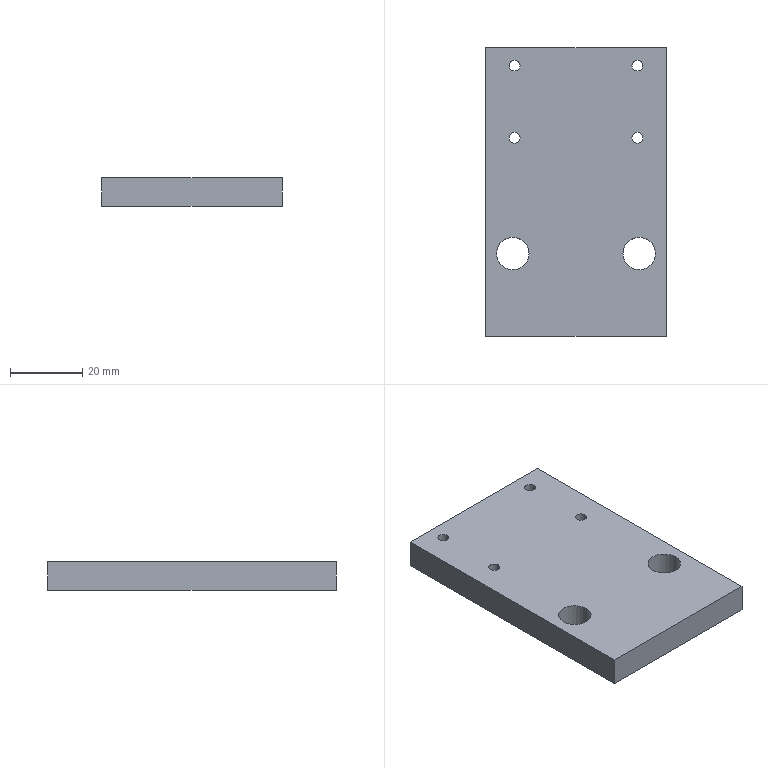Part | STEP file | X77b-01018 | 1 solid | 18 faces | box 50 x 80 x 8 mm | volume 30756 mm3 | cylinder 12 | plane 6 | commonest cylinder face diameters 3 x8 9 x4
STEP:
#1=CARTESIAN_POINT('',(54.163,-91.578,0.));
#2=VERTEX_POINT('',#1);
#3=CARTESIAN_POINT('',(57.163,-91.578,0.));
#4=VERTEX_POINT('',#3);
#5=CARTESIAN_POINT('',(55.663,-91.578,0.));
#6=DIRECTION('',(0.,0.,1.));
#7=DIRECTION('',(1.,0.,0.));
#8=AXIS2_PLACEMENT_3D('',#5,#6,#7);
#9=CIRCLE('',#8,1.5);
#10=EDGE_CURVE('',#2,#4,#9,.T.);
#11=ORIENTED_EDGE('',*,*,#10,.F.);
#12=CARTESIAN_POINT('',(54.163,-91.578,8.));
#13=VERTEX_POINT('',#12);
#14=CARTESIAN_POINT('',(54.163,-91.578,8.));
#15=DIRECTION('',(0.,0.,1.));
#16=VECTOR('',#15,1000.);
#17=LINE('',#14,#16);
#18=EDGE_CURVE('',#2,#13,#17,.T.);
#19=ORIENTED_EDGE('',*,*,#18,.T.);
#20=CARTESIAN_POINT('',(57.163,-91.578,8.));
#21=VERTEX_POINT('',#20);
#22=CARTESIAN_POINT('',(55.663,-91.578,8.));
#23=DIRECTION('',(0.,0.,1.));
#24=DIRECTION('',(1.,0.,0.));
#25=AXIS2_PLACEMENT_3D('',#22,#23,#24);
#26=CIRCLE('',#25,1.5);
#27=EDGE_CURVE('',#13,#21,#26,.T.);
#28=ORIENTED_EDGE('',*,*,#27,.T.);
#29=CARTESIAN_POINT('',(57.163,-91.578,8.));
#30=DIRECTION('',(0.,0.,1.));
#31=VECTOR('',#30,1000.);
#32=LINE('',#29,#31);
#33=EDGE_CURVE('',#4,#21,#32,.T.);
#34=ORIENTED_EDGE('',*,*,#33,.F.);
#35=EDGE_LOOP('',(#11,#19,#28,#34));
#36=FACE_OUTER_BOUND('',#35,.T.);
#37=CARTESIAN_POINT('',(55.663,-91.578,8.));
#38=DIRECTION('',(0.,0.,1.));
#39=DIRECTION('',(1.,0.,0.));
#40=AXIS2_PLACEMENT_3D('',#37,#38,#39);
#41=CYLINDRICAL_SURFACE('',#40,1.5);
#42=ADVANCED_FACE('',(#36),#41,.F.);
#43=CARTESIAN_POINT('',(54.163,-71.578,0.));
#44=VERTEX_POINT('',#43);
#45=CARTESIAN_POINT('',(57.163,-71.578,0.));
#46=VERTEX_POINT('',#45);
#47=CARTESIAN_POINT('',(55.663,-71.578,0.));
#48=DIRECTION('',(0.,0.,1.));
#49=DIRECTION('',(1.,0.,0.));
#50=AXIS2_PLACEMENT_3D('',#47,#48,#49);
#51=CIRCLE('',#50,1.5);
#52=EDGE_CURVE('',#44,#46,#51,.T.);
#53=ORIENTED_EDGE('',*,*,#52,.F.);
#54=CARTESIAN_POINT('',(54.163,-71.578,8.));
#55=VERTEX_POINT('',#54);
#56=CARTESIAN_POINT('',(54.163,-71.578,8.));
#57=DIRECTION('',(0.,0.,1.));
#58=VECTOR('',#57,1000.);
#59=LINE('',#56,#58);
#60=EDGE_CURVE('',#44,#55,#59,.T.);
#61=ORIENTED_EDGE('',*,*,#60,.T.);
#62=CARTESIAN_POINT('',(57.163,-71.578,8.));
#63=VERTEX_POINT('',#62);
#64=CARTESIAN_POINT('',(55.663,-71.578,8.));
#65=DIRECTION('',(0.,0.,1.));
#66=DIRECTION('',(1.,0.,0.));
#67=AXIS2_PLACEMENT_3D('',#64,#65,#66);
#68=CIRCLE('',#67,1.5);
#69=EDGE_CURVE('',#55,#63,#68,.T.);
#70=ORIENTED_EDGE('',*,*,#69,.T.);
#71=CARTESIAN_POINT('',(57.163,-71.578,8.));
#72=DIRECTION('',(0.,0.,1.));
#73=VECTOR('',#72,1000.);
#74=LINE('',#71,#73);
#75=EDGE_CURVE('',#46,#63,#74,.T.);
#76=ORIENTED_EDGE('',*,*,#75,.F.);
#77=EDGE_LOOP('',(#53,#61,#70,#76));
#78=FACE_OUTER_BOUND('',#77,.T.);
#79=CARTESIAN_POINT('',(55.663,-71.578,8.));
#80=DIRECTION('',(0.,0.,1.));
#81=DIRECTION('',(1.,0.,0.));
#82=AXIS2_PLACEMENT_3D('',#79,#80,#81);
#83=CYLINDRICAL_SURFACE('',#82,1.5);
#84=ADVANCED_FACE('',(#78),#83,.F.);
#85=CARTESIAN_POINT('',(88.163,-91.578,0.));
#86=VERTEX_POINT('',#85);
#87=CARTESIAN_POINT('',(91.163,-91.578,0.));
#88=VERTEX_POINT('',#87);
#89=CARTESIAN_POINT('',(89.663,-91.578,0.));
#90=DIRECTION('',(0.,0.,1.));
#91=DIRECTION('',(1.,0.,0.));
#92=AXIS2_PLACEMENT_3D('',#89,#90,#91);
#93=CIRCLE('',#92,1.5);
#94=EDGE_CURVE('',#86,#88,#93,.T.);
#95=ORIENTED_EDGE('',*,*,#94,.F.);
#96=CARTESIAN_POINT('',(88.163,-91.578,8.));
#97=VERTEX_POINT('',#96);
#98=CARTESIAN_POINT('',(88.163,-91.578,8.));
#99=DIRECTION('',(0.,0.,1.));
#100=VECTOR('',#99,1000.);
#101=LINE('',#98,#100);
#102=EDGE_CURVE('',#86,#97,#101,.T.);
#103=ORIENTED_EDGE('',*,*,#102,.T.);
#104=CARTESIAN_POINT('',(91.163,-91.578,8.));
#105=VERTEX_POINT('',#104);
#106=CARTESIAN_POINT('',(89.663,-91.578,8.));
#107=DIRECTION('',(0.,0.,1.));
#108=DIRECTION('',(1.,0.,0.));
#109=AXIS2_PLACEMENT_3D('',#106,#107,#108);
#110=CIRCLE('',#109,1.5);
#111=EDGE_CURVE('',#97,#105,#110,.T.);
#112=ORIENTED_EDGE('',*,*,#111,.T.);
#113=CARTESIAN_POINT('',(91.163,-91.578,8.));
#114=DIRECTION('',(0.,0.,1.));
#115=VECTOR('',#114,1000.);
#116=LINE('',#113,#115);
#117=EDGE_CURVE('',#88,#105,#116,.T.);
#118=ORIENTED_EDGE('',*,*,#117,.F.);
#119=EDGE_LOOP('',(#95,#103,#112,#118));
#120=FACE_OUTER_BOUND('',#119,.T.);
#121=CARTESIAN_POINT('',(89.663,-91.578,8.));
#122=DIRECTION('',(0.,0.,1.));
#123=DIRECTION('',(1.,0.,0.));
#124=AXIS2_PLACEMENT_3D('',#121,#122,#123);
#125=CYLINDRICAL_SURFACE('',#124,1.5);
#126=ADVANCED_FACE('',(#120),#125,.F.);
#127=CARTESIAN_POINT('',(88.163,-71.578,0.));
#128=VERTEX_POINT('',#127);
#129=CARTESIAN_POINT('',(91.163,-71.578,0.));
#130=VERTEX_POINT('',#129);
#131=CARTESIAN_POINT('',(89.663,-71.578,0.));
#132=DIRECTION('',(0.,0.,1.));
#133=DIRECTION('',(1.,0.,0.));
#134=AXIS2_PLACEMENT_3D('',#131,#132,#133);
#135=CIRCLE('',#134,1.5);
#136=EDGE_CURVE('',#128,#130,#135,.T.);
#137=ORIENTED_EDGE('',*,*,#136,.F.);
#138=CARTESIAN_POINT('',(88.163,-71.578,8.));
#139=VERTEX_POINT('',#138);
#140=CARTESIAN_POINT('',(88.163,-71.578,8.));
#141=DIRECTION('',(0.,0.,1.));
#142=VECTOR('',#141,1000.);
#143=LINE('',#140,#142);
#144=EDGE_CURVE('',#128,#139,#143,.T.);
#145=ORIENTED_EDGE('',*,*,#144,.T.);
#146=CARTESIAN_POINT('',(91.163,-71.578,8.));
#147=VERTEX_POINT('',#146);
#148=CARTESIAN_POINT('',(89.663,-71.578,8.));
#149=DIRECTION('',(0.,0.,1.));
#150=DIRECTION('',(1.,0.,0.));
#151=AXIS2_PLACEMENT_3D('',#148,#149,#150);
#152=CIRCLE('',#151,1.5);
#153=EDGE_CURVE('',#139,#147,#152,.T.);
#154=ORIENTED_EDGE('',*,*,#153,.T.);
#155=CARTESIAN_POINT('',(91.163,-71.578,8.));
#156=DIRECTION('',(0.,0.,1.));
#157=VECTOR('',#156,1000.);
#158=LINE('',#155,#157);
#159=EDGE_CURVE('',#130,#147,#158,.T.);
#160=ORIENTED_EDGE('',*,*,#159,.F.);
#161=EDGE_LOOP('',(#137,#145,#154,#160));
#162=FACE_OUTER_BOUND('',#161,.T.);
#163=CARTESIAN_POINT('',(89.663,-71.578,8.));
#164=DIRECTION('',(0.,0.,1.));
#165=DIRECTION('',(1.,0.,0.));
#166=AXIS2_PLACEMENT_3D('',#163,#164,#165);
#167=CYLINDRICAL_SURFACE('',#166,1.5);
#168=ADVANCED_FACE('',(#162),#167,.F.);
#169=CARTESIAN_POINT('',(85.663,-123.626,0.));
#170=VERTEX_POINT('',#169);
#171=CARTESIAN_POINT('',(94.663,-123.626,0.));
#172=VERTEX_POINT('',#171);
#173=CARTESIAN_POINT('',(90.163,-123.626,0.));
#174=DIRECTION('',(0.,0.,1.));
#175=DIRECTION('',(1.,0.,0.));
#176=AXIS2_PLACEMENT_3D('',#173,#174,#175);
#177=CIRCLE('',#176,4.5);
#178=EDGE_CURVE('',#170,#172,#177,.T.);
#179=ORIENTED_EDGE('',*,*,#178,.F.);
#180=CARTESIAN_POINT('',(85.663,-123.626,8.));
#181=VERTEX_POINT('',#180);
#182=CARTESIAN_POINT('',(85.663,-123.626,8.));
#183=DIRECTION('',(0.,0.,1.));
#184=VECTOR('',#183,1000.);
#185=LINE('',#182,#184);
#186=EDGE_CURVE('',#170,#181,#185,.T.);
#187=ORIENTED_EDGE('',*,*,#186,.T.);
#188=CARTESIAN_POINT('',(94.663,-123.626,8.));
#189=VERTEX_POINT('',#188);
#190=CARTESIAN_POINT('',(90.163,-123.626,8.));
#191=DIRECTION('',(0.,0.,1.));
#192=DIRECTION('',(1.,0.,0.));
#193=AXIS2_PLACEMENT_3D('',#190,#191,#192);
#194=CIRCLE('',#193,4.5);
#195=EDGE_CURVE('',#181,#189,#194,.T.);
#196=ORIENTED_EDGE('',*,*,#195,.T.);
#197=CARTESIAN_POINT('',(94.663,-123.626,8.));
#198=DIRECTION('',(0.,0.,1.));
#199=VECTOR('',#198,1000.);
#200=LINE('',#197,#199);
#201=EDGE_CURVE('',#172,#189,#200,.T.);
#202=ORIENTED_EDGE('',*,*,#201,.F.);
#203=EDGE_LOOP('',(#179,#187,#196,#202));
#204=FACE_OUTER_BOUND('',#203,.T.);
#205=CARTESIAN_POINT('',(90.163,-123.626,8.));
#206=DIRECTION('',(0.,0.,1.));
#207=DIRECTION('',(1.,0.,0.));
#208=AXIS2_PLACEMENT_3D('',#205,#206,#207);
#209=CYLINDRICAL_SURFACE('',#208,4.5);
#210=ADVANCED_FACE('',(#204),#209,.F.);
#211=CARTESIAN_POINT('',(50.663,-123.626,0.));
#212=VERTEX_POINT('',#211);
#213=CARTESIAN_POINT('',(59.663,-123.626,0.));
#214=VERTEX_POINT('',#213);
#215=CARTESIAN_POINT('',(55.163,-123.626,0.));
#216=DIRECTION('',(0.,0.,1.));
#217=DIRECTION('',(1.,0.,0.));
#218=AXIS2_PLACEMENT_3D('',#215,#216,#217);
#219=CIRCLE('',#218,4.5);
#220=EDGE_CURVE('',#212,#214,#219,.T.);
#221=ORIENTED_EDGE('',*,*,#220,.F.);
#222=CARTESIAN_POINT('',(50.663,-123.626,8.));
#223=VERTEX_POINT('',#222);
#224=CARTESIAN_POINT('',(50.663,-123.626,8.));
#225=DIRECTION('',(0.,0.,1.));
#226=VECTOR('',#225,1000.);
#227=LINE('',#224,#226);
#228=EDGE_CURVE('',#212,#223,#227,.T.);
#229=ORIENTED_EDGE('',*,*,#228,.T.);
#230=CARTESIAN_POINT('',(59.663,-123.626,8.));
#231=VERTEX_POINT('',#230);
#232=CARTESIAN_POINT('',(55.163,-123.626,8.));
#233=DIRECTION('',(0.,0.,1.));
#234=DIRECTION('',(1.,0.,0.));
#235=AXIS2_PLACEMENT_3D('',#232,#233,#234);
#236=CIRCLE('',#235,4.5);
#237=EDGE_CURVE('',#223,#231,#236,.T.);
#238=ORIENTED_EDGE('',*,*,#237,.T.);
#239=CARTESIAN_POINT('',(59.663,-123.626,8.));
#240=DIRECTION('',(0.,0.,1.));
#241=VECTOR('',#240,1000.);
#242=LINE('',#239,#241);
#243=EDGE_CURVE('',#214,#231,#242,.T.);
#244=ORIENTED_EDGE('',*,*,#243,.F.);
#245=EDGE_LOOP('',(#221,#229,#238,#244));
#246=FACE_OUTER_BOUND('',#245,.T.);
#247=CARTESIAN_POINT('',(55.163,-123.626,8.));
#248=DIRECTION('',(0.,0.,1.));
#249=DIRECTION('',(1.,0.,0.));
#250=AXIS2_PLACEMENT_3D('',#247,#248,#249);
#251=CYLINDRICAL_SURFACE('',#250,4.5);
#252=ADVANCED_FACE('',(#246),#251,.F.);
#253=CARTESIAN_POINT('',(47.663,-66.578,0.));
#254=VERTEX_POINT('',#253);
#255=CARTESIAN_POINT('',(47.663,-146.578,0.));
#256=VERTEX_POINT('',#255);
#257=CARTESIAN_POINT('',(47.663,-66.578,0.));
#258=DIRECTION('',(0.,-1.,0.));
#259=VECTOR('',#258,1000.);
#260=LINE('',#257,#259);
#261=EDGE_CURVE('',#254,#256,#260,.T.);
#262=ORIENTED_EDGE('',*,*,#261,.T.);
#263=CARTESIAN_POINT('',(47.663,-146.578,8.));
#264=VERTEX_POINT('',#263);
#265=CARTESIAN_POINT('',(47.663,-146.578,8.));
#266=DIRECTION('',(0.,0.,-1.));
#267=VECTOR('',#266,1000.);
#268=LINE('',#265,#267);
#269=EDGE_CURVE('',#264,#256,#268,.T.);
#270=ORIENTED_EDGE('',*,*,#269,.F.);
#271=CARTESIAN_POINT('',(47.663,-66.578,8.));
#272=VERTEX_POINT('',#271);
#273=CARTESIAN_POINT('',(47.663,-66.578,8.));
#274=DIRECTION('',(0.,-1.,0.));
#275=VECTOR('',#274,1000.);
#276=LINE('',#273,#275);
#277=EDGE_CURVE('',#272,#264,#276,.T.);
#278=ORIENTED_EDGE('',*,*,#277,.F.);
#279=CARTESIAN_POINT('',(47.663,-66.578,8.));
#280=DIRECTION('',(0.,0.,-1.));
#281=VECTOR('',#280,1000.);
#282=LINE('',#279,#281);
#283=EDGE_CURVE('',#272,#254,#282,.T.);
#284=ORIENTED_EDGE('',*,*,#283,.T.);
#285=EDGE_LOOP('',(#262,#270,#278,#284));
#286=FACE_OUTER_BOUND('',#285,.T.);
#287=CARTESIAN_POINT('',(47.663,-66.578,8.));
#288=DIRECTION('',(1.,0.,0.));
#289=DIRECTION('',(0.,1.,0.));
#290=AXIS2_PLACEMENT_3D('',#287,#288,#289);
#291=PLANE('',#290);
#292=ADVANCED_FACE('',(#286),#291,.F.);
#293=CARTESIAN_POINT('',(97.663,-146.578,0.));
#294=VERTEX_POINT('',#293);
#295=CARTESIAN_POINT('',(47.663,-146.578,0.));
#296=DIRECTION('',(1.,0.,0.));
#297=VECTOR('',#296,1000.);
#298=LINE('',#295,#297);
#299=EDGE_CURVE('',#256,#294,#298,.T.);
#300=ORIENTED_EDGE('',*,*,#299,.T.);
#301=CARTESIAN_POINT('',(97.663,-146.578,8.));
#302=VERTEX_POINT('',#301);
#303=CARTESIAN_POINT('',(97.663,-146.578,8.));
#304=DIRECTION('',(0.,0.,-1.));
#305=VECTOR('',#304,1000.);
#306=LINE('',#303,#305);
#307=EDGE_CURVE('',#302,#294,#306,.T.);
#308=ORIENTED_EDGE('',*,*,#307,.F.);
#309=CARTESIAN_POINT('',(47.663,-146.578,8.));
#310=DIRECTION('',(1.,0.,0.));
#311=VECTOR('',#310,1000.);
#312=LINE('',#309,#311);
#313=EDGE_CURVE('',#264,#302,#312,.T.);
#314=ORIENTED_EDGE('',*,*,#313,.F.);
#315=ORIENTED_EDGE('',*,*,#269,.T.);
#316=EDGE_LOOP('',(#300,#308,#314,#315));
#317=FACE_OUTER_BOUND('',#316,.T.);
#318=CARTESIAN_POINT('',(47.663,-146.578,8.));
#319=DIRECTION('',(0.,1.,0.));
#320=DIRECTION('',(0.,0.,1.));
#321=AXIS2_PLACEMENT_3D('',#318,#319,#320);
#322=PLANE('',#321);
#323=ADVANCED_FACE('',(#317),#322,.F.);
#324=CARTESIAN_POINT('',(97.663,-66.578,0.));
#325=VERTEX_POINT('',#324);
#326=CARTESIAN_POINT('',(97.663,-66.578,0.));
#327=DIRECTION('',(0.,1.,0.));
#328=VECTOR('',#327,1000.);
#329=LINE('',#326,#328);
#330=EDGE_CURVE('',#294,#325,#329,.T.);
#331=ORIENTED_EDGE('',*,*,#330,.T.);
#332=CARTESIAN_POINT('',(97.663,-66.578,8.));
#333=VERTEX_POINT('',#332);
#334=CARTESIAN_POINT('',(97.663,-66.578,8.));
#335=DIRECTION('',(0.,0.,-1.));
#336=VECTOR('',#335,1000.);
#337=LINE('',#334,#336);
#338=EDGE_CURVE('',#333,#325,#337,.T.);
#339=ORIENTED_EDGE('',*,*,#338,.F.);
#340=CARTESIAN_POINT('',(97.663,-66.578,8.));
#341=DIRECTION('',(0.,1.,0.));
#342=VECTOR('',#341,1000.);
#343=LINE('',#340,#342);
#344=EDGE_CURVE('',#302,#333,#343,.T.);
#345=ORIENTED_EDGE('',*,*,#344,.F.);
#346=ORIENTED_EDGE('',*,*,#307,.T.);
#347=EDGE_LOOP('',(#331,#339,#345,#346));
#348=FACE_OUTER_BOUND('',#347,.T.);
#349=CARTESIAN_POINT('',(97.663,-66.578,8.));
#350=DIRECTION('',(-1.,0.,0.));
#351=DIRECTION('',(0.,0.,1.));
#352=AXIS2_PLACEMENT_3D('',#349,#350,#351);
#353=PLANE('',#352);
#354=ADVANCED_FACE('',(#348),#353,.F.);
#355=CARTESIAN_POINT('',(47.663,-66.578,0.));
#356=DIRECTION('',(-1.,0.,0.));
#357=VECTOR('',#356,1000.);
#358=LINE('',#355,#357);
#359=EDGE_CURVE('',#325,#254,#358,.T.);
#360=ORIENTED_EDGE('',*,*,#359,.T.);
#361=ORIENTED_EDGE('',*,*,#283,.F.);
#362=CARTESIAN_POINT('',(47.663,-66.578,8.));
#363=DIRECTION('',(-1.,0.,0.));
#364=VECTOR('',#363,1000.);
#365=LINE('',#362,#364);
#366=EDGE_CURVE('',#333,#272,#365,.T.);
#367=ORIENTED_EDGE('',*,*,#366,.F.);
#368=ORIENTED_EDGE('',*,*,#338,.T.);
#369=EDGE_LOOP('',(#360,#361,#367,#368));
#370=FACE_OUTER_BOUND('',#369,.T.);
#371=CARTESIAN_POINT('',(47.663,-66.578,8.));
#372=DIRECTION('',(0.,-1.,0.));
#373=DIRECTION('',(0.,0.,-1.));
#374=AXIS2_PLACEMENT_3D('',#371,#372,#373);
#375=PLANE('',#374);
#376=ADVANCED_FACE('',(#370),#375,.F.);
#377=CARTESIAN_POINT('',(55.663,-91.578,8.));
#378=DIRECTION('',(0.,0.,1.));
#379=DIRECTION('',(1.,0.,0.));
#380=AXIS2_PLACEMENT_3D('',#377,#378,#379);
#381=CIRCLE('',#380,1.5);
#382=EDGE_CURVE('',#21,#13,#381,.T.);
#383=ORIENTED_EDGE('',*,*,#382,.F.);
#384=ORIENTED_EDGE('',*,*,#27,.F.);
#385=EDGE_LOOP('',(#383,#384));
#386=FACE_BOUND('',#385,.T.);
#387=CARTESIAN_POINT('',(55.663,-71.578,8.));
#388=DIRECTION('',(0.,0.,1.));
#389=DIRECTION('',(1.,0.,0.));
#390=AXIS2_PLACEMENT_3D('',#387,#388,#389);
#391=CIRCLE('',#390,1.5);
#392=EDGE_CURVE('',#63,#55,#391,.T.);
#393=ORIENTED_EDGE('',*,*,#392,.F.);
#394=ORIENTED_EDGE('',*,*,#69,.F.);
#395=EDGE_LOOP('',(#393,#394));
#396=FACE_BOUND('',#395,.T.);
#397=CARTESIAN_POINT('',(89.663,-91.578,8.));
#398=DIRECTION('',(0.,0.,1.));
#399=DIRECTION('',(1.,0.,0.));
#400=AXIS2_PLACEMENT_3D('',#397,#398,#399);
#401=CIRCLE('',#400,1.5);
#402=EDGE_CURVE('',#105,#97,#401,.T.);
#403=ORIENTED_EDGE('',*,*,#402,.F.);
#404=ORIENTED_EDGE('',*,*,#111,.F.);
#405=EDGE_LOOP('',(#403,#404));
#406=FACE_BOUND('',#405,.T.);
#407=CARTESIAN_POINT('',(89.663,-71.578,8.));
#408=DIRECTION('',(0.,0.,1.));
#409=DIRECTION('',(1.,0.,0.));
#410=AXIS2_PLACEMENT_3D('',#407,#408,#409);
#411=CIRCLE('',#410,1.5);
#412=EDGE_CURVE('',#147,#139,#411,.T.);
#413=ORIENTED_EDGE('',*,*,#412,.F.);
#414=ORIENTED_EDGE('',*,*,#153,.F.);
#415=EDGE_LOOP('',(#413,#414));
#416=FACE_BOUND('',#415,.T.);
#417=CARTESIAN_POINT('',(90.163,-123.626,8.));
#418=DIRECTION('',(0.,0.,1.));
#419=DIRECTION('',(1.,0.,0.));
#420=AXIS2_PLACEMENT_3D('',#417,#418,#419);
#421=CIRCLE('',#420,4.5);
#422=EDGE_CURVE('',#189,#181,#421,.T.);
#423=ORIENTED_EDGE('',*,*,#422,.F.);
#424=ORIENTED_EDGE('',*,*,#195,.F.);
#425=EDGE_LOOP('',(#423,#424));
#426=FACE_BOUND('',#425,.T.);
#427=CARTESIAN_POINT('',(55.163,-123.626,8.));
#428=DIRECTION('',(0.,0.,1.));
#429=DIRECTION('',(1.,0.,0.));
#430=AXIS2_PLACEMENT_3D('',#427,#428,#429);
#431=CIRCLE('',#430,4.5);
#432=EDGE_CURVE('',#231,#223,#431,.T.);
#433=ORIENTED_EDGE('',*,*,#432,.F.);
#434=ORIENTED_EDGE('',*,*,#237,.F.);
#435=EDGE_LOOP('',(#433,#434));
#436=FACE_BOUND('',#435,.T.);
#437=ORIENTED_EDGE('',*,*,#277,.T.);
#438=ORIENTED_EDGE('',*,*,#313,.T.);
#439=ORIENTED_EDGE('',*,*,#344,.T.);
#440=ORIENTED_EDGE('',*,*,#366,.T.);
#441=EDGE_LOOP('',(#437,#438,#439,#440));
#442=FACE_OUTER_BOUND('',#441,.T.);
#443=CARTESIAN_POINT('',(47.663,-146.578,8.));
#444=DIRECTION('',(0.,0.,1.));
#445=DIRECTION('',(1.,0.,0.));
#446=AXIS2_PLACEMENT_3D('',#443,#444,#445);
#447=PLANE('',#446);
#448=ADVANCED_FACE('',(#386,#396,#406,#416,#426,#436,#442),#447,.T.);
#449=CARTESIAN_POINT('',(55.663,-91.578,0.));
#450=DIRECTION('',(0.,0.,1.));
#451=DIRECTION('',(1.,0.,0.));
#452=AXIS2_PLACEMENT_3D('',#449,#450,#451);
#453=CIRCLE('',#452,1.5);
#454=EDGE_CURVE('',#4,#2,#453,.T.);
#455=ORIENTED_EDGE('',*,*,#454,.T.);
#456=ORIENTED_EDGE('',*,*,#10,.T.);
#457=EDGE_LOOP('',(#455,#456));
#458=FACE_BOUND('',#457,.T.);
#459=CARTESIAN_POINT('',(55.663,-71.578,0.));
#460=DIRECTION('',(0.,0.,1.));
#461=DIRECTION('',(1.,0.,0.));
#462=AXIS2_PLACEMENT_3D('',#459,#460,#461);
#463=CIRCLE('',#462,1.5);
#464=EDGE_CURVE('',#46,#44,#463,.T.);
#465=ORIENTED_EDGE('',*,*,#464,.T.);
#466=ORIENTED_EDGE('',*,*,#52,.T.);
#467=EDGE_LOOP('',(#465,#466));
#468=FACE_BOUND('',#467,.T.);
#469=CARTESIAN_POINT('',(89.663,-91.578,0.));
#470=DIRECTION('',(0.,0.,1.));
#471=DIRECTION('',(1.,0.,0.));
#472=AXIS2_PLACEMENT_3D('',#469,#470,#471);
#473=CIRCLE('',#472,1.5);
#474=EDGE_CURVE('',#88,#86,#473,.T.);
#475=ORIENTED_EDGE('',*,*,#474,.T.);
#476=ORIENTED_EDGE('',*,*,#94,.T.);
#477=EDGE_LOOP('',(#475,#476));
#478=FACE_BOUND('',#477,.T.);
#479=CARTESIAN_POINT('',(89.663,-71.578,0.));
#480=DIRECTION('',(0.,0.,1.));
#481=DIRECTION('',(1.,0.,0.));
#482=AXIS2_PLACEMENT_3D('',#479,#480,#481);
#483=CIRCLE('',#482,1.5);
#484=EDGE_CURVE('',#130,#128,#483,.T.);
#485=ORIENTED_EDGE('',*,*,#484,.T.);
#486=ORIENTED_EDGE('',*,*,#136,.T.);
#487=EDGE_LOOP('',(#485,#486));
#488=FACE_BOUND('',#487,.T.);
#489=CARTESIAN_POINT('',(90.163,-123.626,0.));
#490=DIRECTION('',(0.,0.,1.));
#491=DIRECTION('',(1.,0.,0.));
#492=AXIS2_PLACEMENT_3D('',#489,#490,#491);
#493=CIRCLE('',#492,4.5);
#494=EDGE_CURVE('',#172,#170,#493,.T.);
#495=ORIENTED_EDGE('',*,*,#494,.T.);
#496=ORIENTED_EDGE('',*,*,#178,.T.);
#497=EDGE_LOOP('',(#495,#496));
#498=FACE_BOUND('',#497,.T.);
#499=CARTESIAN_POINT('',(55.163,-123.626,0.));
#500=DIRECTION('',(0.,0.,1.));
#501=DIRECTION('',(1.,0.,0.));
#502=AXIS2_PLACEMENT_3D('',#499,#500,#501);
#503=CIRCLE('',#502,4.5);
#504=EDGE_CURVE('',#214,#212,#503,.T.);
#505=ORIENTED_EDGE('',*,*,#504,.T.);
#506=ORIENTED_EDGE('',*,*,#220,.T.);
#507=EDGE_LOOP('',(#505,#506));
#508=FACE_BOUND('',#507,.T.);
#509=ORIENTED_EDGE('',*,*,#261,.F.);
#510=ORIENTED_EDGE('',*,*,#359,.F.);
#511=ORIENTED_EDGE('',*,*,#330,.F.);
#512=ORIENTED_EDGE('',*,*,#299,.F.);
#513=EDGE_LOOP('',(#509,#510,#511,#512));
#514=FACE_OUTER_BOUND('',#513,.T.);
#515=CARTESIAN_POINT('',(47.663,-146.578,0.));
#516=DIRECTION('',(0.,0.,1.));
#517=DIRECTION('',(1.,0.,0.));
#518=AXIS2_PLACEMENT_3D('',#515,#516,#517);
#519=PLANE('',#518);
#520=ADVANCED_FACE('',(#458,#468,#478,#488,#498,#508,#514),#519,.F.);
#521=ORIENTED_EDGE('',*,*,#228,.F.);
#522=ORIENTED_EDGE('',*,*,#504,.F.);
#523=ORIENTED_EDGE('',*,*,#243,.T.);
#524=ORIENTED_EDGE('',*,*,#432,.T.);
#525=EDGE_LOOP('',(#521,#522,#523,#524));
#526=FACE_OUTER_BOUND('',#525,.T.);
#527=CARTESIAN_POINT('',(55.163,-123.626,8.));
#528=DIRECTION('',(0.,0.,1.));
#529=DIRECTION('',(1.,0.,0.));
#530=AXIS2_PLACEMENT_3D('',#527,#528,#529);
#531=CYLINDRICAL_SURFACE('',#530,4.5);
#532=ADVANCED_FACE('',(#526),#531,.F.);
#533=ORIENTED_EDGE('',*,*,#186,.F.);
#534=ORIENTED_EDGE('',*,*,#494,.F.);
#535=ORIENTED_EDGE('',*,*,#201,.T.);
#536=ORIENTED_EDGE('',*,*,#422,.T.);
#537=EDGE_LOOP('',(#533,#534,#535,#536));
#538=FACE_OUTER_BOUND('',#537,.T.);
#539=CARTESIAN_POINT('',(90.163,-123.626,8.));
#540=DIRECTION('',(0.,0.,1.));
#541=DIRECTION('',(1.,0.,0.));
#542=AXIS2_PLACEMENT_3D('',#539,#540,#541);
#543=CYLINDRICAL_SURFACE('',#542,4.5);
#544=ADVANCED_FACE('',(#538),#543,.F.);
#545=ORIENTED_EDGE('',*,*,#144,.F.);
#546=ORIENTED_EDGE('',*,*,#484,.F.);
#547=ORIENTED_EDGE('',*,*,#159,.T.);
#548=ORIENTED_EDGE('',*,*,#412,.T.);
#549=EDGE_LOOP('',(#545,#546,#547,#548));
#550=FACE_OUTER_BOUND('',#549,.T.);
#551=CARTESIAN_POINT('',(89.663,-71.578,8.));
#552=DIRECTION('',(0.,0.,1.));
#553=DIRECTION('',(1.,0.,0.));
#554=AXIS2_PLACEMENT_3D('',#551,#552,#553);
#555=CYLINDRICAL_SURFACE('',#554,1.5);
#556=ADVANCED_FACE('',(#550),#555,.F.);
#557=ORIENTED_EDGE('',*,*,#102,.F.);
#558=ORIENTED_EDGE('',*,*,#474,.F.);
#559=ORIENTED_EDGE('',*,*,#117,.T.);
#560=ORIENTED_EDGE('',*,*,#402,.T.);
#561=EDGE_LOOP('',(#557,#558,#559,#560));
#562=FACE_OUTER_BOUND('',#561,.T.);
#563=CARTESIAN_POINT('',(89.663,-91.578,8.));
#564=DIRECTION('',(0.,0.,1.));
#565=DIRECTION('',(1.,0.,0.));
#566=AXIS2_PLACEMENT_3D('',#563,#564,#565);
#567=CYLINDRICAL_SURFACE('',#566,1.5);
#568=ADVANCED_FACE('',(#562),#567,.F.);
#569=ORIENTED_EDGE('',*,*,#60,.F.);
#570=ORIENTED_EDGE('',*,*,#464,.F.);
#571=ORIENTED_EDGE('',*,*,#75,.T.);
#572=ORIENTED_EDGE('',*,*,#392,.T.);
#573=EDGE_LOOP('',(#569,#570,#571,#572));
#574=FACE_OUTER_BOUND('',#573,.T.);
#575=CARTESIAN_POINT('',(55.663,-71.578,8.));
#576=DIRECTION('',(0.,0.,1.));
#577=DIRECTION('',(1.,0.,0.));
#578=AXIS2_PLACEMENT_3D('',#575,#576,#577);
#579=CYLINDRICAL_SURFACE('',#578,1.5);
#580=ADVANCED_FACE('',(#574),#579,.F.);
#581=ORIENTED_EDGE('',*,*,#18,.F.);
#582=ORIENTED_EDGE('',*,*,#454,.F.);
#583=ORIENTED_EDGE('',*,*,#33,.T.);
#584=ORIENTED_EDGE('',*,*,#382,.T.);
#585=EDGE_LOOP('',(#581,#582,#583,#584));
#586=FACE_OUTER_BOUND('',#585,.T.);
#587=CARTESIAN_POINT('',(55.663,-91.578,8.));
#588=DIRECTION('',(0.,0.,1.));
#589=DIRECTION('',(1.,0.,0.));
#590=AXIS2_PLACEMENT_3D('',#587,#588,#589);
#591=CYLINDRICAL_SURFACE('',#590,1.5);
#592=ADVANCED_FACE('',(#586),#591,.F.);
#593=CLOSED_SHELL('',(#42,#84,#126,#168,#210,#252,#292,#323,#354,#376,#448,#520,#532,#544,#556,#568,#580,#592));
#594=MANIFOLD_SOLID_BREP('',#593);
#595=CARTESIAN_POINT('',(0.,0.,0.));
#596=DIRECTION('',(0.,0.,1.));
#597=DIRECTION('',(1.,0.,0.));
#598=AXIS2_PLACEMENT_3D('',#595,#596,#597);
#599=(LENGTH_UNIT()NAMED_UNIT(*)SI_UNIT(.MILLI.,.METRE.));
#600=UNCERTAINTY_MEASURE_WITH_UNIT(LENGTH_MEASURE(0.00001),#599,'','');
#601=(NAMED_UNIT(*)PLANE_ANGLE_UNIT()SI_UNIT($,.RADIAN.));
#602=(NAMED_UNIT(*)SI_UNIT($,.STERADIAN.)SOLID_ANGLE_UNIT());
#603=(GEOMETRIC_REPRESENTATION_CONTEXT(3)GLOBAL_UNCERTAINTY_ASSIGNED_CONTEXT((#600))GLOBAL_UNIT_ASSIGNED_CONTEXT((#599,#601,#602))REPRESENTATION_CONTEXT('',''));
#604=ADVANCED_BREP_SHAPE_REPRESENTATION('',(#594,#598),#603);